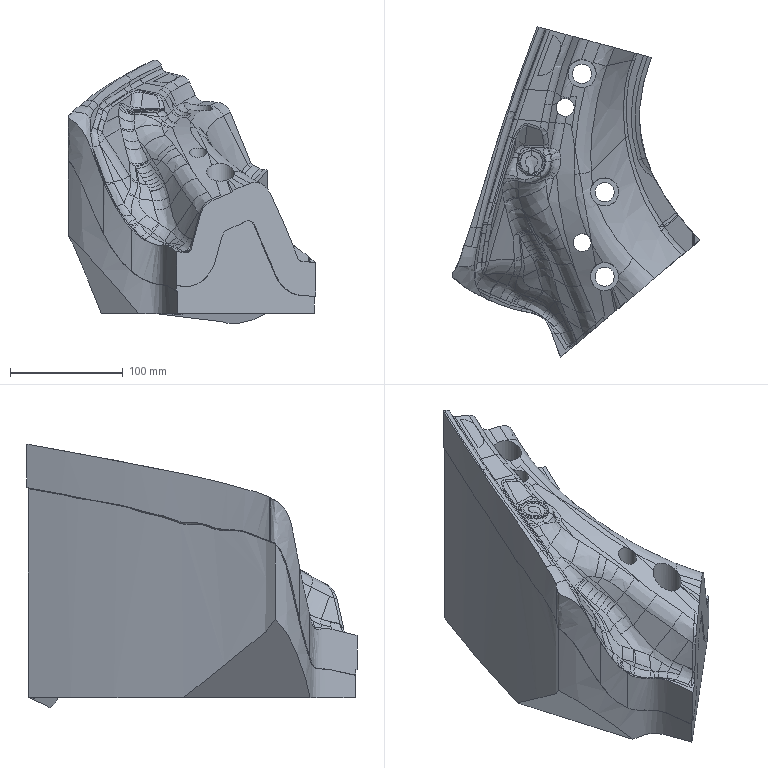Part | NX | features solid 2 | 1 solid | 294 faces | volume 4674740 mm3 | spline 265 | plane 19 | cylinder 10 | commonest cylinder face diameters 25 x5 17 x3 16 x2